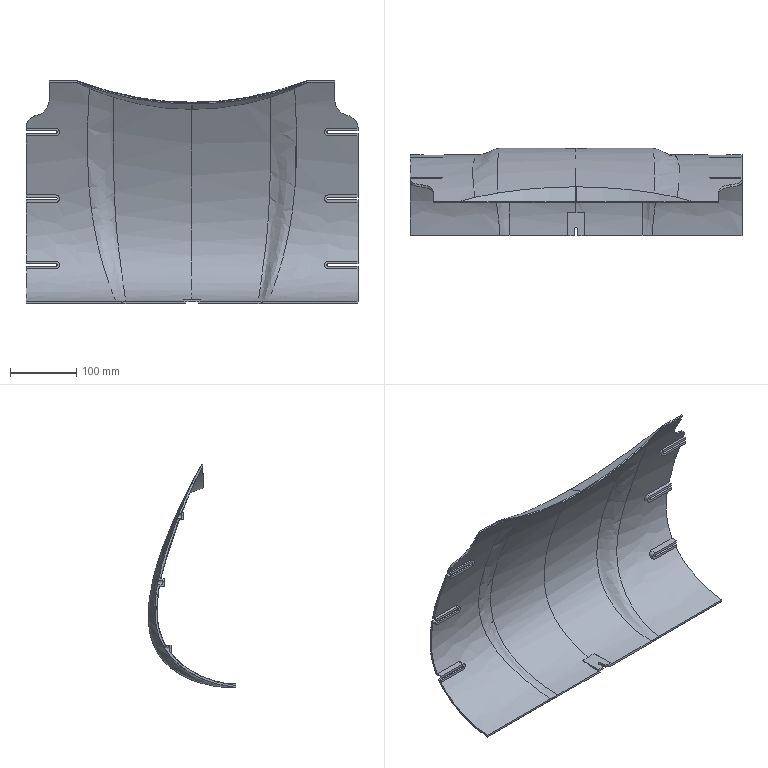Part | STEP file | MOTOR COVER Z | 1 solid | 128 faces | box 500 x 131.956 x 336.482 mm | volume 623732 mm3 | plane 81 | cylinder 21 | spline 20 | cone 6 | commonest cylinder face diameters 3.5 x6 6.5 x6 11 x6 48 x2 4.5 x1